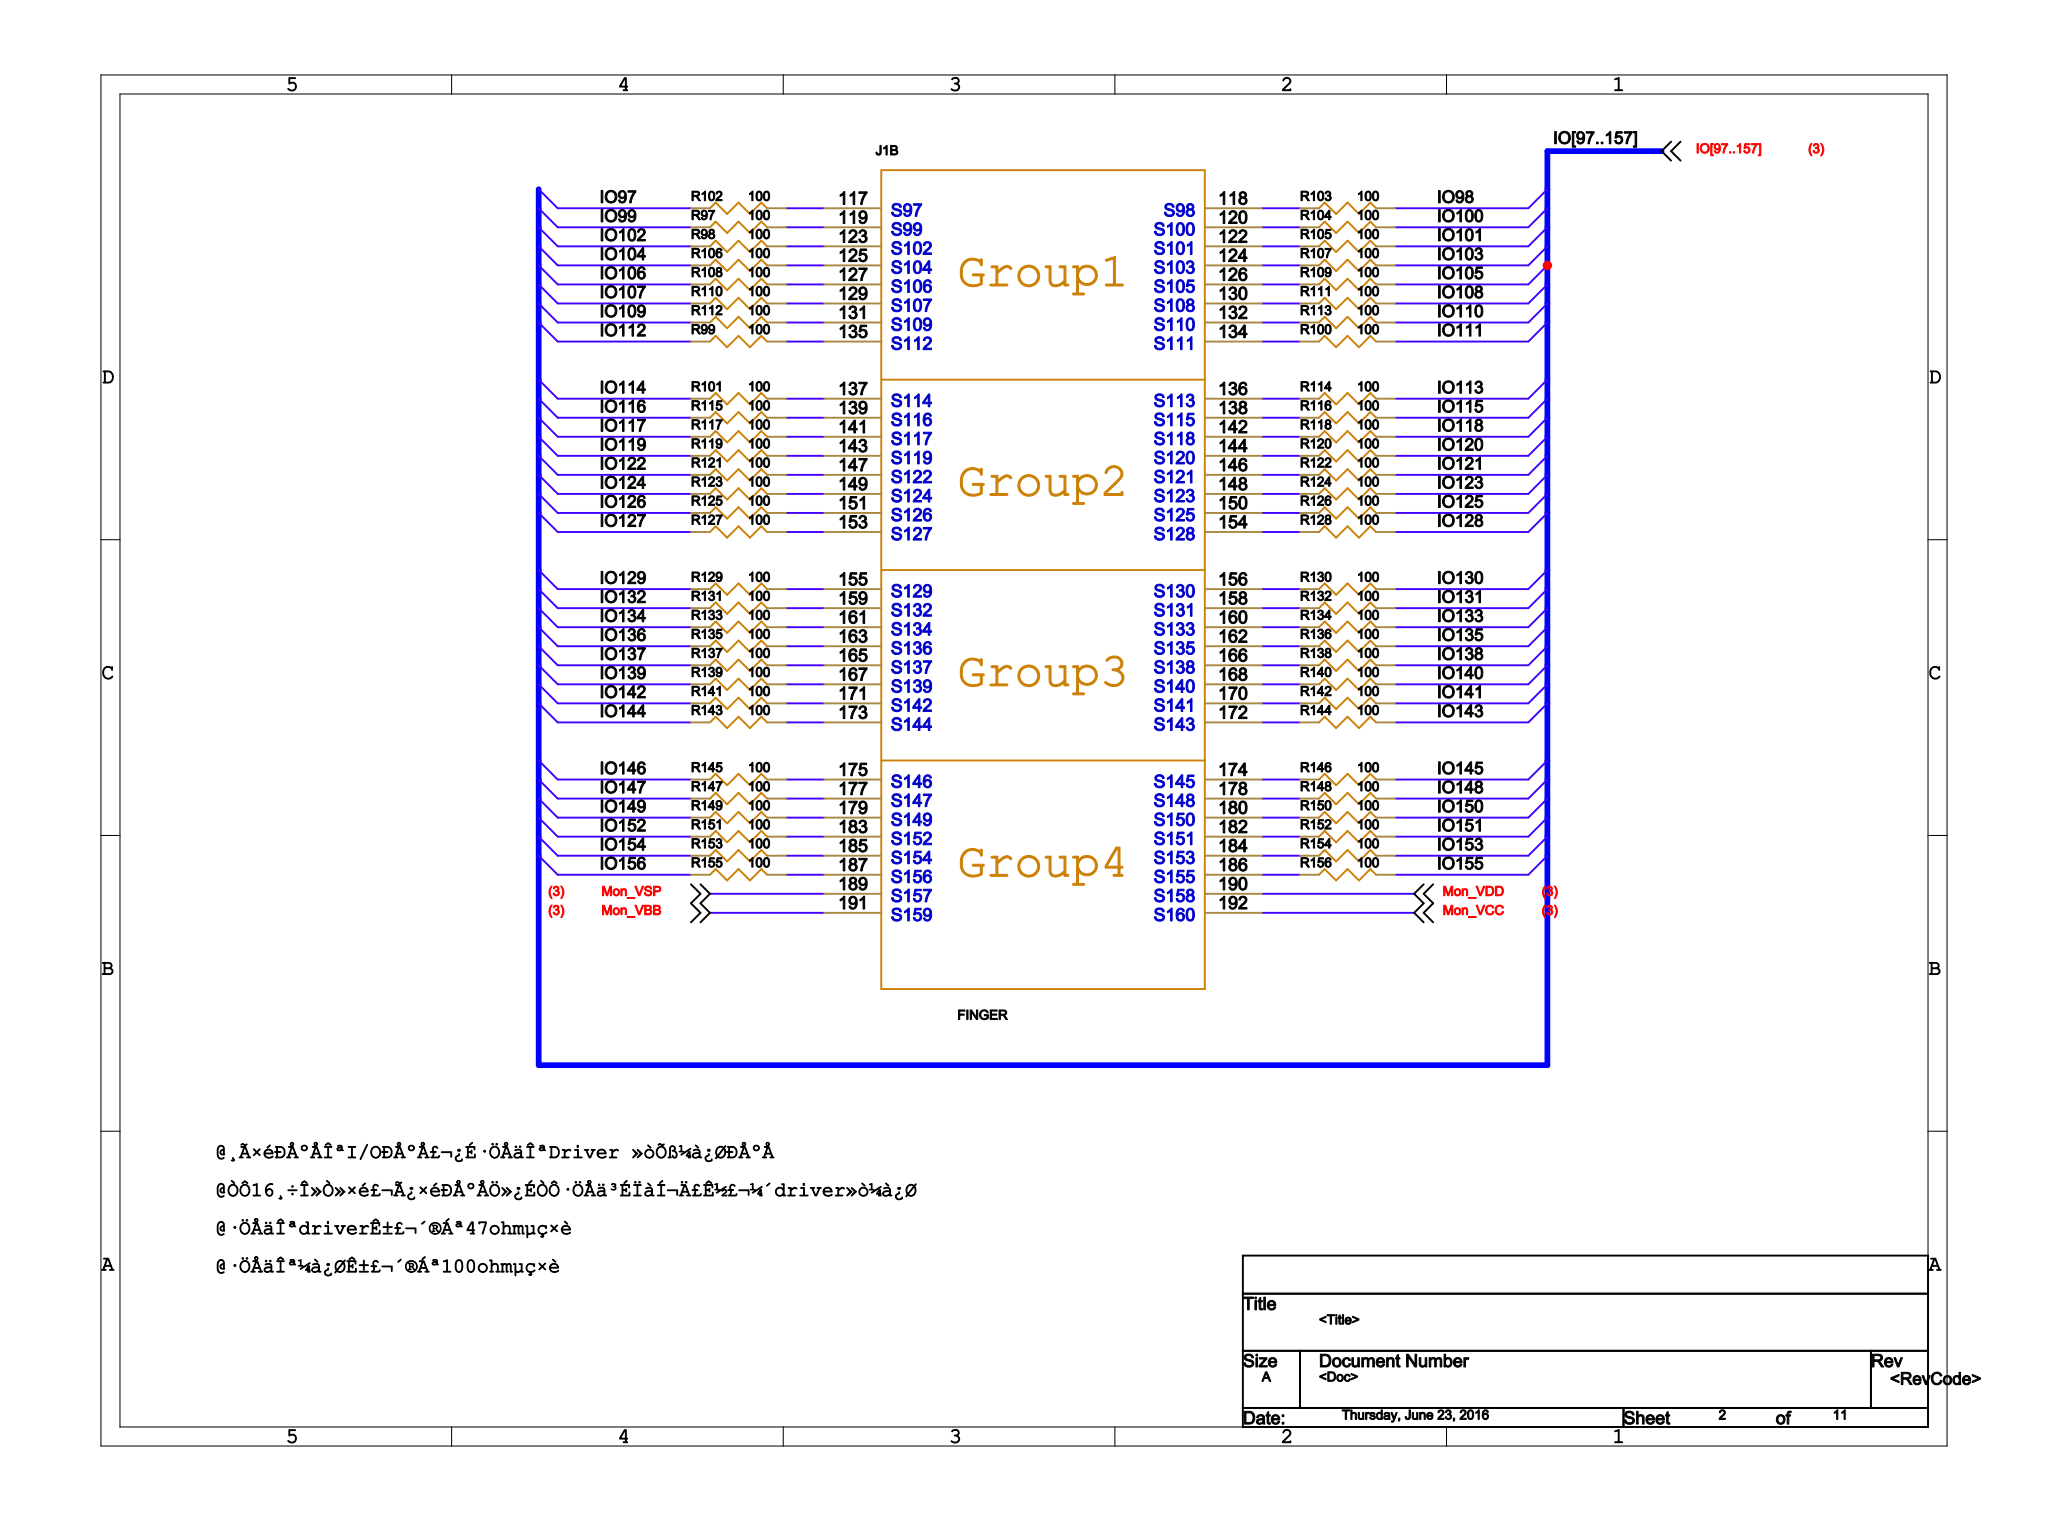Circuit board | Cadence Allegro | 531 parts | 624 nets | one sheet of the schematic
Parts on this sheet (reference | value | footprint):
J1 | FINGER | FINGER
R97 | 100 | RES2-400-100
R98 | 100 | RES2-400-100
R99 | 100 | RES2-400-100
R100 | 100 | RES2-400-100
R101 | 100 | RES2-400-100
R102 | 100 | RES2-400-100
R103 | 100 | RES2-400-100
R104 | 100 | RES2-400-100
R105 | 100 | RES2-400-100
R106 | 100 | RES2-400-100
R107 | 100 | RES2-400-100
R108 | 100 | RES2-400-100
R109 | 100 | RES2-400-100
R110 | 100 | RES2-400-100
R111 | 100 | RES2-400-100
R112 | 100 | RES2-400-100
R113 | 100 | RES2-400-100
R114 | 100 | RES2-400-100
R115 | 100 | RES2-400-100
R116 | 100 | RES2-400-100
R117 | 100 | RES2-400-100
R118 | 100 | RES2-400-100
R119 | 100 | RES2-400-100
R120 | 100 | RES2-400-100
R121 | 100 | RES2-400-100
R122 | 100 | RES2-400-100
R123 | 100 | RES2-400-100
R124 | 100 | RES2-400-100
R125 | 100 | RES2-400-100
R126 | 100 | RES2-400-100
R127 | 100 | RES2-400-100
R128 | 100 | RES2-400-100
R129 | 100 | RES2-400-100
R130 | 100 | RES2-400-100
R131 | 100 | RES2-400-100
R132 | 100 | RES2-400-100
R133 | 100 | RES2-400-100
R134 | 100 | RES2-400-100
R135 | 100 | RES2-400-100
R136 | 100 | RES2-400-100
R137 | 100 | RES2-400-100
R138 | 100 | RES2-400-100
R139 | 100 | RES2-400-100
R140 | 100 | RES2-400-100
R141 | 100 | RES2-400-100
R142 | 100 | RES2-400-100
R143 | 100 | RES2-400-100
R144 | 100 | RES2-400-100
R145 | 100 | RES2-400-100
R146 | 100 | RES2-400-100
R147 | 100 | RES2-400-100
R148 | 100 | RES2-400-100
R149 | 100 | RES2-400-100
R150 | 100 | RES2-400-100
R151 | 100 | RES2-400-100
R152 | 100 | RES2-400-100
R153 | 100 | RES2-400-100
R154 | 100 | RES2-400-100
R155 | 100 | RES2-400-100
R156 | 100 | RES2-400-100
Nets of these parts (net: part-pin ...):
IO145: R146-2
IO151: R152-2
IO152: R151-1
IO146: R145-1
IO147: R147-1
IO148: R148-2
IO149: R149-1
IO150: R150-2
N6403590: R100-1 J1-134
IO111: R100-2
IO114: R101-1
N6394641: R101-2 J1-137
IO109: R112-1
N6394199: R112-2 J1-131
N6403278: R113-1 J1-132
IO110: R113-2
N6404109: R114-1 J1-136
IO113: R114-2
IO116: R115-1
N6394737: R115-2 J1-139
N6404286: R116-1 J1-138
IO115: R116-2
IO117: R117-1
N6394835: R117-2 J1-141
N6404465: R118-1 J1-142
IO118: R118-2
IO119: R119-1
N6394935: R119-2 J1-143
N6404646: R120-1 J1-144
IO120: R120-2
IO122: R121-1
N6395037: R121-2 J1-147
N6404829: R122-1 J1-146
IO121: R122-2
IO124: R123-1
N6395141: R123-2 J1-149
N6405014: R124-1 J1-148
IO123: R124-2
IO126: R125-1
N6395247: R125-2 J1-151
N6405201: R126-1 J1-150
IO125: R126-2
IO127: R127-1
N6395355: R127-2 J1-153
N6405390: R128-1 J1-154
IO128: R128-2
IO129: R129-1
N6395691: R129-2 J1-155
N6405969: R130-1 J1-156
IO130: R130-2
IO132: R131-1
N6395807: R131-2 J1-159
N6406166: R132-1 J1-158
IO131: R132-2
IO134: R133-1
N6395925: R133-2 J1-161
N6406365: R134-1 J1-160
IO133: R134-2
IO136: R135-1
N6396045: R135-2 J1-163
N6406566: R136-1 J1-162
IO135: R136-2
IO137: R137-1
N6396167: R137-2 J1-165
N6406769: R138-1 J1-166
IO138: R138-2
IO139: R139-1
N6396291: R139-2 J1-167
N6406974: R140-1 J1-168
IO140: R140-2
IO142: R141-1
N6396417: R141-2 J1-171
N6407181: R142-1 J1-170
IO141: R142-2
IO144: R143-1
N6396545: R143-2 J1-173
N6407390: R144-1 J1-172
IO143: R144-2
N6396941: R145-2 J1-175
N6408029: R146-1 J1-174
N6397077: R147-2 J1-177
N6408246: R148-1 J1-178
N6397215: R149-2 J1-179
N6408465: R150-1 J1-180
N6397355: R151-2 J1-183
N6408686: R152-1 J1-182
IO154: R153-1
N6397497: R153-2 J1-185
N6408909: R154-1 J1-184
IO153: R154-2
IO156: R155-1
N6397641: R155-2 J1-187
N6409134: R156-1 J1-186
IO155: R156-2
IO112: R99-1
N6394349: R99-2 J1-135
N4509297: R104-1 J1-120
IO100: R104-2
IO102: R98-1
N4417347: R98-2 J1-123
N4142381: R105-1 J1-122
IO101: R105-2
IO104: R106-1
N4417468: R106-2 J1-125
N4509895: R107-1 J1-124
IO103: R107-2
IO106: R108-1
N4417590: R108-2 J1-127
N4142389: R109-1 J1-126
IO105: R109-2
IO107: R110-1
N4417713: R110-2 J1-129
N4400458: R111-1 J1-130
IO108: R111-2
IO97: R102-1
N4415654: R102-2 J1-117
N4142373: R103-1 J1-118
IO98: R103-2
IO99: R97-1
N4417111: R97-2 J1-119